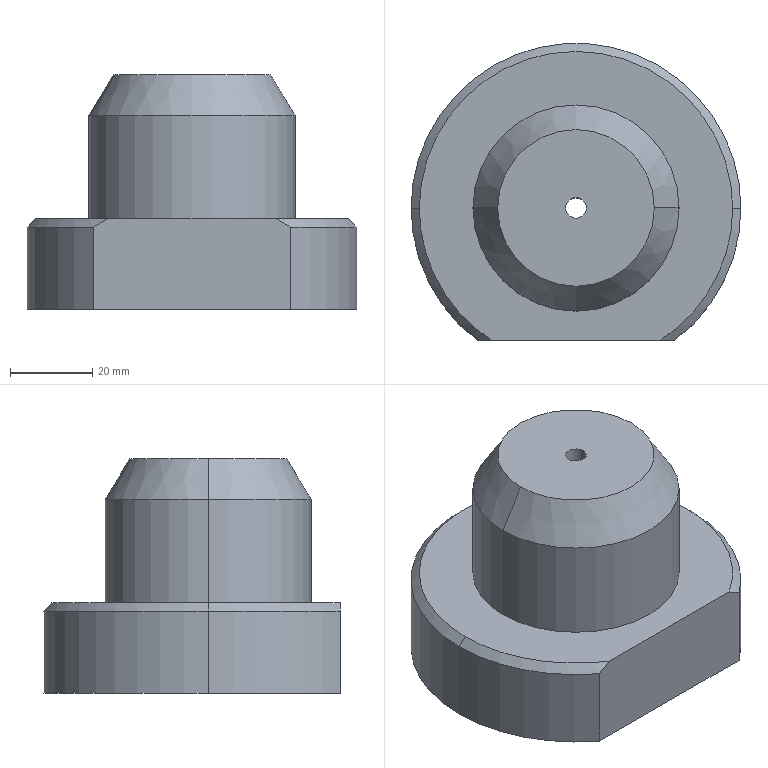Part | SolidWorks | features Chamfer 2, ICE 2, Extrusion 1, HoleWzd 1 | 1 solid | 16 faces | box 80 x 72 x 57 mm | volume 167700 mm3 | cylinder 7 | cone 5 | plane 4 | commonest cylinder face diameters 80 x3 5 x2 50 x2
STEP:
#1=CARTESIAN_POINT('',(2.5,0.,35.));
#2=VERTEX_POINT('',#1);
#3=CARTESIAN_POINT('',(-2.5,0.,35.));
#4=VERTEX_POINT('',#3);
#5=CARTESIAN_POINT('',(0.,0.,35.));
#6=DIRECTION('',(0.,0.,-1.));
#7=DIRECTION('',(-1.,0.,0.));
#8=AXIS2_PLACEMENT_3D('',#5,#6,#7);
#9=CIRCLE('',#8,2.5);
#10=EDGE_CURVE('',#2,#4,#9,.T.);
#11=ORIENTED_EDGE('',*,*,#10,.F.);
#12=CARTESIAN_POINT('',(2.5,0.,-22.));
#13=VERTEX_POINT('',#12);
#14=CARTESIAN_POINT('',(2.5,0.,-22.));
#15=DIRECTION('',(0.,0.,-1.));
#16=VECTOR('',#15,1000.);
#17=LINE('',#14,#16);
#18=EDGE_CURVE('',#2,#13,#17,.T.);
#19=ORIENTED_EDGE('',*,*,#18,.T.);
#20=CARTESIAN_POINT('',(-2.5,0.,-22.));
#21=VERTEX_POINT('',#20);
#22=CARTESIAN_POINT('',(0.,0.,-22.));
#23=DIRECTION('',(0.,0.,-1.));
#24=DIRECTION('',(-1.,0.,0.));
#25=AXIS2_PLACEMENT_3D('',#22,#23,#24);
#26=CIRCLE('',#25,2.5);
#27=EDGE_CURVE('',#13,#21,#26,.T.);
#28=ORIENTED_EDGE('',*,*,#27,.T.);
#29=CARTESIAN_POINT('',(-2.5,0.,-22.));
#30=DIRECTION('',(0.,0.,-1.));
#31=VECTOR('',#30,1000.);
#32=LINE('',#29,#31);
#33=EDGE_CURVE('',#4,#21,#32,.T.);
#34=ORIENTED_EDGE('',*,*,#33,.F.);
#35=EDGE_LOOP('',(#11,#19,#28,#34));
#36=FACE_OUTER_BOUND('',#35,.T.);
#37=CARTESIAN_POINT('',(0.,0.,-22.));
#38=DIRECTION('',(0.,0.,-1.));
#39=DIRECTION('',(-1.,0.,0.));
#40=AXIS2_PLACEMENT_3D('',#37,#38,#39);
#41=CYLINDRICAL_SURFACE('',#40,2.5);
#42=ADVANCED_FACE('',(#36),#41,.F.);
#43=CARTESIAN_POINT('',(38.,0.,0.));
#44=VERTEX_POINT('',#43);
#45=CARTESIAN_POINT('',(-38.,0.,0.));
#46=VERTEX_POINT('',#45);
#47=CARTESIAN_POINT('',(0.,0.,0.));
#48=DIRECTION('',(0.,0.,1.));
#49=DIRECTION('',(-1.,0.,0.));
#50=AXIS2_PLACEMENT_3D('',#47,#48,#49);
#51=CIRCLE('',#50,38.);
#52=EDGE_CURVE('',#44,#46,#51,.T.);
#53=ORIENTED_EDGE('',*,*,#52,.F.);
#54=CARTESIAN_POINT('',(40.,0.,-2.));
#55=VERTEX_POINT('',#54);
#56=CARTESIAN_POINT('',(40.,0.,-2.));
#57=DIRECTION('',(0.7071,0.,-0.7071));
#58=VECTOR('',#57,1000.);
#59=LINE('',#56,#58);
#60=EDGE_CURVE('',#44,#55,#59,.T.);
#61=ORIENTED_EDGE('',*,*,#60,.T.);
#62=CARTESIAN_POINT('',(-40.,0.,-2.));
#63=VERTEX_POINT('',#62);
#64=CARTESIAN_POINT('',(0.,0.,-2.));
#65=DIRECTION('',(0.,0.,-1.));
#66=DIRECTION('',(-1.,0.,0.));
#67=AXIS2_PLACEMENT_3D('',#64,#65,#66);
#68=CIRCLE('',#67,40.);
#69=EDGE_CURVE('',#63,#55,#68,.T.);
#70=ORIENTED_EDGE('',*,*,#69,.F.);
#71=CARTESIAN_POINT('',(-40.,0.,-2.));
#72=DIRECTION('',(-0.7071,0.,-0.7071));
#73=VECTOR('',#72,1000.);
#74=LINE('',#71,#73);
#75=EDGE_CURVE('',#46,#63,#74,.T.);
#76=ORIENTED_EDGE('',*,*,#75,.F.);
#77=EDGE_LOOP('',(#53,#61,#70,#76));
#78=FACE_OUTER_BOUND('',#77,.T.);
#79=CARTESIAN_POINT('',(0.,0.,-2.));
#80=DIRECTION('',(0.,0.,-1.));
#81=DIRECTION('',(-1.,0.,0.));
#82=AXIS2_PLACEMENT_3D('',#79,#80,#81);
#83=CONICAL_SURFACE('',#82,40.,0.7854);
#84=ADVANCED_FACE('',(#78),#83,.T.);
#85=CARTESIAN_POINT('',(-20.494,-32.,0.));
#86=VERTEX_POINT('',#85);
#87=CARTESIAN_POINT('',(0.,0.,0.));
#88=DIRECTION('',(0.,0.,1.));
#89=DIRECTION('',(-1.,0.,0.));
#90=AXIS2_PLACEMENT_3D('',#87,#88,#89);
#91=CIRCLE('',#90,38.);
#92=EDGE_CURVE('',#46,#86,#91,.T.);
#93=ORIENTED_EDGE('',*,*,#92,.F.);
#94=ORIENTED_EDGE('',*,*,#75,.T.);
#95=CARTESIAN_POINT('',(-24.,-32.,-2.));
#96=VERTEX_POINT('',#95);
#97=CARTESIAN_POINT('',(0.,0.,-2.));
#98=DIRECTION('',(0.,0.,-1.));
#99=DIRECTION('',(-1.,0.,0.));
#100=AXIS2_PLACEMENT_3D('',#97,#98,#99);
#101=CIRCLE('',#100,40.);
#102=EDGE_CURVE('',#96,#63,#101,.T.);
#103=ORIENTED_EDGE('',*,*,#102,.F.);
#104=CARTESIAN_POINT('',(-20.494,-32.,0.));
#105=CARTESIAN_POINT('',(-21.678,-32.,-0.6389));
#106=CARTESIAN_POINT('',(-22.846,-32.,-1.308));
#107=CARTESIAN_POINT('',(-24.,-32.,-2.));
#108=B_SPLINE_CURVE_WITH_KNOTS('',3,(#104,#105,#106,#107),.UNSPECIFIED.,.F.,.F.,(4,4),(0.,0.004036),.UNSPECIFIED.);
#109=EDGE_CURVE('',#86,#96,#108,.T.);
#110=ORIENTED_EDGE('',*,*,#109,.F.);
#111=EDGE_LOOP('',(#93,#94,#103,#110));
#112=FACE_OUTER_BOUND('',#111,.T.);
#113=CARTESIAN_POINT('',(0.,0.,-2.));
#114=DIRECTION('',(0.,0.,-1.));
#115=DIRECTION('',(-1.,0.,0.));
#116=AXIS2_PLACEMENT_3D('',#113,#114,#115);
#117=CONICAL_SURFACE('',#116,40.,0.7854);
#118=ADVANCED_FACE('',(#112),#117,.T.);
#119=CARTESIAN_POINT('',(-40.,0.,-22.));
#120=VERTEX_POINT('',#119);
#121=CARTESIAN_POINT('',(40.,0.,-22.));
#122=VERTEX_POINT('',#121);
#123=CARTESIAN_POINT('',(0.,0.,-22.));
#124=DIRECTION('',(0.,0.,-1.));
#125=DIRECTION('',(-1.,0.,0.));
#126=AXIS2_PLACEMENT_3D('',#123,#124,#125);
#127=CIRCLE('',#126,40.);
#128=EDGE_CURVE('',#120,#122,#127,.T.);
#129=ORIENTED_EDGE('',*,*,#128,.F.);
#130=CARTESIAN_POINT('',(-40.,0.,-22.));
#131=DIRECTION('',(0.,0.,1.));
#132=VECTOR('',#131,1000.);
#133=LINE('',#130,#132);
#134=EDGE_CURVE('',#120,#63,#133,.T.);
#135=ORIENTED_EDGE('',*,*,#134,.T.);
#136=ORIENTED_EDGE('',*,*,#69,.T.);
#137=CARTESIAN_POINT('',(40.,0.,-22.));
#138=DIRECTION('',(0.,0.,1.));
#139=VECTOR('',#138,1000.);
#140=LINE('',#137,#139);
#141=EDGE_CURVE('',#122,#55,#140,.T.);
#142=ORIENTED_EDGE('',*,*,#141,.F.);
#143=EDGE_LOOP('',(#129,#135,#136,#142));
#144=FACE_OUTER_BOUND('',#143,.T.);
#145=CARTESIAN_POINT('',(0.,0.,-22.));
#146=DIRECTION('',(0.,0.,1.));
#147=DIRECTION('',(1.,0.,0.));
#148=AXIS2_PLACEMENT_3D('',#145,#146,#147);
#149=CYLINDRICAL_SURFACE('',#148,40.);
#150=ADVANCED_FACE('',(#144),#149,.T.);
#151=CARTESIAN_POINT('',(24.,-32.,-22.));
#152=VERTEX_POINT('',#151);
#153=CARTESIAN_POINT('',(0.,0.,-22.));
#154=DIRECTION('',(0.,0.,-1.));
#155=DIRECTION('',(-1.,0.,0.));
#156=AXIS2_PLACEMENT_3D('',#153,#154,#155);
#157=CIRCLE('',#156,40.);
#158=EDGE_CURVE('',#122,#152,#157,.T.);
#159=ORIENTED_EDGE('',*,*,#158,.F.);
#160=ORIENTED_EDGE('',*,*,#141,.T.);
#161=CARTESIAN_POINT('',(24.,-32.,-2.));
#162=VERTEX_POINT('',#161);
#163=CARTESIAN_POINT('',(0.,0.,-2.));
#164=DIRECTION('',(0.,0.,-1.));
#165=DIRECTION('',(-1.,0.,0.));
#166=AXIS2_PLACEMENT_3D('',#163,#164,#165);
#167=CIRCLE('',#166,40.);
#168=EDGE_CURVE('',#55,#162,#167,.T.);
#169=ORIENTED_EDGE('',*,*,#168,.T.);
#170=CARTESIAN_POINT('',(24.,-32.,-22.));
#171=DIRECTION('',(0.,0.,-1.));
#172=VECTOR('',#171,1000.);
#173=LINE('',#170,#172);
#174=EDGE_CURVE('',#162,#152,#173,.T.);
#175=ORIENTED_EDGE('',*,*,#174,.T.);
#176=EDGE_LOOP('',(#159,#160,#169,#175));
#177=FACE_OUTER_BOUND('',#176,.T.);
#178=CARTESIAN_POINT('',(0.,0.,-22.));
#179=DIRECTION('',(0.,0.,1.));
#180=DIRECTION('',(1.,0.,0.));
#181=AXIS2_PLACEMENT_3D('',#178,#179,#180);
#182=CYLINDRICAL_SURFACE('',#181,40.);
#183=ADVANCED_FACE('',(#177),#182,.T.);
#184=CARTESIAN_POINT('',(19.,0.,35.));
#185=VERTEX_POINT('',#184);
#186=CARTESIAN_POINT('',(-19.,0.,35.));
#187=VERTEX_POINT('',#186);
#188=CARTESIAN_POINT('',(0.,0.,35.));
#189=DIRECTION('',(0.,0.,1.));
#190=DIRECTION('',(1.,0.,0.));
#191=AXIS2_PLACEMENT_3D('',#188,#189,#190);
#192=CIRCLE('',#191,19.);
#193=EDGE_CURVE('',#185,#187,#192,.T.);
#194=ORIENTED_EDGE('',*,*,#193,.F.);
#195=CARTESIAN_POINT('',(25.,0.,25.));
#196=VERTEX_POINT('',#195);
#197=CARTESIAN_POINT('',(19.,0.,35.));
#198=DIRECTION('',(0.5145,0.,-0.8575));
#199=VECTOR('',#198,1000.);
#200=LINE('',#197,#199);
#201=EDGE_CURVE('',#185,#196,#200,.T.);
#202=ORIENTED_EDGE('',*,*,#201,.T.);
#203=CARTESIAN_POINT('',(-25.,0.,25.));
#204=VERTEX_POINT('',#203);
#205=CARTESIAN_POINT('',(0.,0.,25.));
#206=DIRECTION('',(0.,0.,-1.));
#207=DIRECTION('',(1.,0.,0.));
#208=AXIS2_PLACEMENT_3D('',#205,#206,#207);
#209=CIRCLE('',#208,25.);
#210=EDGE_CURVE('',#204,#196,#209,.T.);
#211=ORIENTED_EDGE('',*,*,#210,.F.);
#212=CARTESIAN_POINT('',(-19.,0.,35.));
#213=DIRECTION('',(-0.5145,0.,-0.8575));
#214=VECTOR('',#213,1000.);
#215=LINE('',#212,#214);
#216=EDGE_CURVE('',#187,#204,#215,.T.);
#217=ORIENTED_EDGE('',*,*,#216,.F.);
#218=EDGE_LOOP('',(#194,#202,#211,#217));
#219=FACE_OUTER_BOUND('',#218,.T.);
#220=CARTESIAN_POINT('',(0.,0.,35.));
#221=DIRECTION('',(0.,0.,-1.));
#222=DIRECTION('',(-1.,0.,0.));
#223=AXIS2_PLACEMENT_3D('',#220,#221,#222);
#224=CONICAL_SURFACE('',#223,19.,0.5404);
#225=ADVANCED_FACE('',(#219),#224,.T.);
#226=ORIENTED_EDGE('',*,*,#210,.T.);
#227=CARTESIAN_POINT('',(25.,0.,0.));
#228=VERTEX_POINT('',#227);
#229=CARTESIAN_POINT('',(25.,0.,35.));
#230=DIRECTION('',(0.,0.,-1.));
#231=VECTOR('',#230,1000.);
#232=LINE('',#229,#231);
#233=EDGE_CURVE('',#196,#228,#232,.T.);
#234=ORIENTED_EDGE('',*,*,#233,.T.);
#235=CARTESIAN_POINT('',(-25.,0.,0.));
#236=VERTEX_POINT('',#235);
#237=CARTESIAN_POINT('',(0.,0.,0.));
#238=DIRECTION('',(0.,0.,1.));
#239=DIRECTION('',(1.,0.,0.));
#240=AXIS2_PLACEMENT_3D('',#237,#238,#239);
#241=CIRCLE('',#240,25.);
#242=EDGE_CURVE('',#228,#236,#241,.T.);
#243=ORIENTED_EDGE('',*,*,#242,.T.);
#244=CARTESIAN_POINT('',(-25.,0.,35.));
#245=DIRECTION('',(0.,0.,-1.));
#246=VECTOR('',#245,1000.);
#247=LINE('',#244,#246);
#248=EDGE_CURVE('',#204,#236,#247,.T.);
#249=ORIENTED_EDGE('',*,*,#248,.F.);
#250=EDGE_LOOP('',(#226,#234,#243,#249));
#251=FACE_OUTER_BOUND('',#250,.T.);
#252=CARTESIAN_POINT('',(0.,0.,35.));
#253=DIRECTION('',(0.,0.,-1.));
#254=DIRECTION('',(-1.,0.,0.));
#255=AXIS2_PLACEMENT_3D('',#252,#253,#254);
#256=CYLINDRICAL_SURFACE('',#255,25.);
#257=ADVANCED_FACE('',(#251),#256,.T.);
#258=ORIENTED_EDGE('',*,*,#233,.F.);
#259=CARTESIAN_POINT('',(0.,0.,25.));
#260=DIRECTION('',(0.,0.,-1.));
#261=DIRECTION('',(1.,0.,0.));
#262=AXIS2_PLACEMENT_3D('',#259,#260,#261);
#263=CIRCLE('',#262,25.);
#264=EDGE_CURVE('',#196,#204,#263,.T.);
#265=ORIENTED_EDGE('',*,*,#264,.T.);
#266=ORIENTED_EDGE('',*,*,#248,.T.);
#267=CARTESIAN_POINT('',(0.,0.,0.));
#268=DIRECTION('',(0.,0.,1.));
#269=DIRECTION('',(1.,0.,0.));
#270=AXIS2_PLACEMENT_3D('',#267,#268,#269);
#271=CIRCLE('',#270,25.);
#272=EDGE_CURVE('',#236,#228,#271,.T.);
#273=ORIENTED_EDGE('',*,*,#272,.T.);
#274=EDGE_LOOP('',(#258,#265,#266,#273));
#275=FACE_OUTER_BOUND('',#274,.T.);
#276=CARTESIAN_POINT('',(0.,0.,35.));
#277=DIRECTION('',(0.,0.,-1.));
#278=DIRECTION('',(-1.,0.,0.));
#279=AXIS2_PLACEMENT_3D('',#276,#277,#278);
#280=CYLINDRICAL_SURFACE('',#279,25.);
#281=ADVANCED_FACE('',(#275),#280,.T.);
#282=CARTESIAN_POINT('',(0.,0.,35.));
#283=DIRECTION('',(0.,0.,-1.));
#284=DIRECTION('',(-1.,0.,0.));
#285=AXIS2_PLACEMENT_3D('',#282,#283,#284);
#286=CIRCLE('',#285,2.5);
#287=EDGE_CURVE('',#4,#2,#286,.T.);
#288=ORIENTED_EDGE('',*,*,#287,.T.);
#289=ORIENTED_EDGE('',*,*,#10,.T.);
#290=EDGE_LOOP('',(#288,#289));
#291=FACE_BOUND('',#290,.T.);
#292=CARTESIAN_POINT('',(0.,0.,35.));
#293=DIRECTION('',(0.,0.,1.));
#294=DIRECTION('',(1.,0.,0.));
#295=AXIS2_PLACEMENT_3D('',#292,#293,#294);
#296=CIRCLE('',#295,19.);
#297=EDGE_CURVE('',#187,#185,#296,.T.);
#298=ORIENTED_EDGE('',*,*,#297,.T.);
#299=ORIENTED_EDGE('',*,*,#193,.T.);
#300=EDGE_LOOP('',(#298,#299));
#301=FACE_OUTER_BOUND('',#300,.T.);
#302=CARTESIAN_POINT('',(0.,0.,35.));
#303=DIRECTION('',(0.,0.,1.));
#304=DIRECTION('',(1.,0.,0.));
#305=AXIS2_PLACEMENT_3D('',#302,#303,#304);
#306=PLANE('',#305);
#307=ADVANCED_FACE('',(#291,#301),#306,.T.);
#308=ORIENTED_EDGE('',*,*,#201,.F.);
#309=ORIENTED_EDGE('',*,*,#297,.F.);
#310=ORIENTED_EDGE('',*,*,#216,.T.);
#311=ORIENTED_EDGE('',*,*,#264,.F.);
#312=EDGE_LOOP('',(#308,#309,#310,#311));
#313=FACE_OUTER_BOUND('',#312,.T.);
#314=CARTESIAN_POINT('',(0.,0.,35.));
#315=DIRECTION('',(0.,0.,-1.));
#316=DIRECTION('',(-1.,0.,0.));
#317=AXIS2_PLACEMENT_3D('',#314,#315,#316);
#318=CONICAL_SURFACE('',#317,19.,0.5404);
#319=ADVANCED_FACE('',(#313),#318,.T.);
#320=ORIENTED_EDGE('',*,*,#134,.F.);
#321=CARTESIAN_POINT('',(-24.,-32.,-22.));
#322=VERTEX_POINT('',#321);
#323=CARTESIAN_POINT('',(0.,0.,-22.));
#324=DIRECTION('',(0.,0.,-1.));
#325=DIRECTION('',(-1.,0.,0.));
#326=AXIS2_PLACEMENT_3D('',#323,#324,#325);
#327=CIRCLE('',#326,40.);
#328=EDGE_CURVE('',#322,#120,#327,.T.);
#329=ORIENTED_EDGE('',*,*,#328,.F.);
#330=CARTESIAN_POINT('',(-24.,-32.,-22.));
#331=DIRECTION('',(0.,0.,1.));
#332=VECTOR('',#331,1000.);
#333=LINE('',#330,#332);
#334=EDGE_CURVE('',#322,#96,#333,.T.);
#335=ORIENTED_EDGE('',*,*,#334,.T.);
#336=ORIENTED_EDGE('',*,*,#102,.T.);
#337=EDGE_LOOP('',(#320,#329,#335,#336));
#338=FACE_OUTER_BOUND('',#337,.T.);
#339=CARTESIAN_POINT('',(0.,0.,-22.));
#340=DIRECTION('',(0.,0.,1.));
#341=DIRECTION('',(1.,0.,0.));
#342=AXIS2_PLACEMENT_3D('',#339,#340,#341);
#343=CYLINDRICAL_SURFACE('',#342,40.);
#344=ADVANCED_FACE('',(#338),#343,.T.);
#345=CARTESIAN_POINT('',(0.,0.,-22.));
#346=DIRECTION('',(0.,0.,-1.));
#347=DIRECTION('',(-1.,0.,0.));
#348=AXIS2_PLACEMENT_3D('',#345,#346,#347);
#349=CIRCLE('',#348,2.5);
#350=EDGE_CURVE('',#21,#13,#349,.T.);
#351=ORIENTED_EDGE('',*,*,#350,.F.);
#352=ORIENTED_EDGE('',*,*,#27,.F.);
#353=EDGE_LOOP('',(#351,#352));
#354=FACE_BOUND('',#353,.T.);
#355=CARTESIAN_POINT('',(-30.,-32.,-22.));
#356=DIRECTION('',(1.,0.,0.));
#357=VECTOR('',#356,1000.);
#358=LINE('',#355,#357);
#359=EDGE_CURVE('',#322,#152,#358,.T.);
#360=ORIENTED_EDGE('',*,*,#359,.F.);
#361=ORIENTED_EDGE('',*,*,#328,.T.);
#362=ORIENTED_EDGE('',*,*,#128,.T.);
#363=ORIENTED_EDGE('',*,*,#158,.T.);
#364=EDGE_LOOP('',(#360,#361,#362,#363));
#365=FACE_OUTER_BOUND('',#364,.T.);
#366=CARTESIAN_POINT('',(0.,0.,-22.));
#367=DIRECTION('',(0.,0.,-1.));
#368=DIRECTION('',(-1.,0.,0.));
#369=AXIS2_PLACEMENT_3D('',#366,#367,#368);
#370=PLANE('',#369);
#371=ADVANCED_FACE('',(#354,#365),#370,.T.);
#372=ORIENTED_EDGE('',*,*,#272,.F.);
#373=ORIENTED_EDGE('',*,*,#242,.F.);
#374=EDGE_LOOP('',(#372,#373));
#375=FACE_BOUND('',#374,.T.);
#376=CARTESIAN_POINT('',(20.494,-32.,0.));
#377=VERTEX_POINT('',#376);
#378=CARTESIAN_POINT('',(0.,-32.,0.));
#379=DIRECTION('',(1.,0.,0.));
#380=VECTOR('',#379,1000.);
#381=LINE('',#378,#380);
#382=EDGE_CURVE('',#86,#377,#381,.T.);
#383=ORIENTED_EDGE('',*,*,#382,.T.);
#384=CARTESIAN_POINT('',(0.,0.,0.));
#385=DIRECTION('',(0.,0.,1.));
#386=DIRECTION('',(-1.,0.,0.));
#387=AXIS2_PLACEMENT_3D('',#384,#385,#386);
#388=CIRCLE('',#387,38.);
#389=EDGE_CURVE('',#377,#44,#388,.T.);
#390=ORIENTED_EDGE('',*,*,#389,.T.);
#391=ORIENTED_EDGE('',*,*,#52,.T.);
#392=ORIENTED_EDGE('',*,*,#92,.T.);
#393=EDGE_LOOP('',(#383,#390,#391,#392));
#394=FACE_OUTER_BOUND('',#393,.T.);
#395=CARTESIAN_POINT('',(0.,0.,0.));
#396=DIRECTION('',(0.,0.,-1.));
#397=DIRECTION('',(-1.,0.,0.));
#398=AXIS2_PLACEMENT_3D('',#395,#396,#397);
#399=PLANE('',#398);
#400=ADVANCED_FACE('',(#375,#394),#399,.F.);
#401=ORIENTED_EDGE('',*,*,#174,.F.);
#402=CARTESIAN_POINT('',(24.,-32.,-2.));
#403=CARTESIAN_POINT('',(22.846,-32.,-1.308));
#404=CARTESIAN_POINT('',(21.678,-32.,-0.6389));
#405=CARTESIAN_POINT('',(20.494,-32.,0.));
#406=B_SPLINE_CURVE_WITH_KNOTS('',3,(#402,#403,#404,#405),.UNSPECIFIED.,.F.,.F.,(4,4),(0.,0.004036),.UNSPECIFIED.);
#407=EDGE_CURVE('',#162,#377,#406,.T.);
#408=ORIENTED_EDGE('',*,*,#407,.T.);
#409=ORIENTED_EDGE('',*,*,#382,.F.);
#410=ORIENTED_EDGE('',*,*,#109,.T.);
#411=ORIENTED_EDGE('',*,*,#334,.F.);
#412=ORIENTED_EDGE('',*,*,#359,.T.);
#413=EDGE_LOOP('',(#401,#408,#409,#410,#411,#412));
#414=FACE_OUTER_BOUND('',#413,.T.);
#415=CARTESIAN_POINT('',(-30.,-32.,68.));
#416=DIRECTION('',(0.,1.,0.));
#417=DIRECTION('',(0.,0.,1.));
#418=AXIS2_PLACEMENT_3D('',#415,#416,#417);
#419=PLANE('',#418);
#420=ADVANCED_FACE('',(#414),#419,.F.);
#421=ORIENTED_EDGE('',*,*,#60,.F.);
#422=ORIENTED_EDGE('',*,*,#389,.F.);
#423=ORIENTED_EDGE('',*,*,#407,.F.);
#424=ORIENTED_EDGE('',*,*,#168,.F.);
#425=EDGE_LOOP('',(#421,#422,#423,#424));
#426=FACE_OUTER_BOUND('',#425,.T.);
#427=CARTESIAN_POINT('',(0.,0.,-2.));
#428=DIRECTION('',(0.,0.,-1.));
#429=DIRECTION('',(-1.,0.,0.));
#430=AXIS2_PLACEMENT_3D('',#427,#428,#429);
#431=CONICAL_SURFACE('',#430,40.,0.7854);
#432=ADVANCED_FACE('',(#426),#431,.T.);
#433=ORIENTED_EDGE('',*,*,#18,.F.);
#434=ORIENTED_EDGE('',*,*,#287,.F.);
#435=ORIENTED_EDGE('',*,*,#33,.T.);
#436=ORIENTED_EDGE('',*,*,#350,.T.);
#437=EDGE_LOOP('',(#433,#434,#435,#436));
#438=FACE_OUTER_BOUND('',#437,.T.);
#439=CARTESIAN_POINT('',(0.,0.,-22.));
#440=DIRECTION('',(0.,0.,-1.));
#441=DIRECTION('',(-1.,0.,0.));
#442=AXIS2_PLACEMENT_3D('',#439,#440,#441);
#443=CYLINDRICAL_SURFACE('',#442,2.5);
#444=ADVANCED_FACE('',(#438),#443,.F.);
#445=CLOSED_SHELL('',(#42,#84,#118,#150,#183,#225,#257,#281,#307,#319,#344,#371,#400,#420,#432,#444));
#446=MANIFOLD_SOLID_BREP('',#445);
#447=CARTESIAN_POINT('',(0.,0.,0.));
#448=DIRECTION('',(0.,0.,1.));
#449=DIRECTION('',(1.,0.,0.));
#450=AXIS2_PLACEMENT_3D('',#447,#448,#449);
#451=(LENGTH_UNIT()NAMED_UNIT(*)SI_UNIT(.MILLI.,.METRE.));
#452=UNCERTAINTY_MEASURE_WITH_UNIT(LENGTH_MEASURE(0.00001),#451,'','');
#453=(NAMED_UNIT(*)PLANE_ANGLE_UNIT()SI_UNIT($,.RADIAN.));
#454=(NAMED_UNIT(*)SI_UNIT($,.STERADIAN.)SOLID_ANGLE_UNIT());
#455=(GEOMETRIC_REPRESENTATION_CONTEXT(3)GLOBAL_UNCERTAINTY_ASSIGNED_CONTEXT((#452))GLOBAL_UNIT_ASSIGNED_CONTEXT((#451,#453,#454))REPRESENTATION_CONTEXT('',''));
#456=ADVANCED_BREP_SHAPE_REPRESENTATION('',(#446,#450),#455);